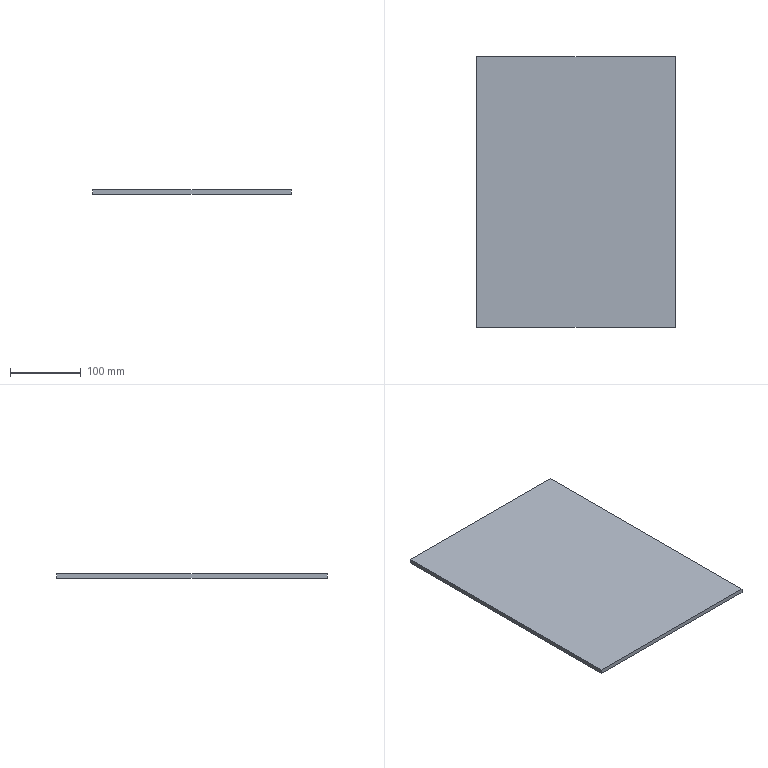Part | STEP file | Drawer | 1 solid | 6 faces | box 280 x 382 x 6 mm | volume 641760 mm3 | plane 6
STEP:
#1=CARTESIAN_POINT('',(0.,0.,0.));
#2=DIRECTION('',(0.,0.,1.));
#3=DIRECTION('',(1.,0.,0.));
#4=AXIS2_PLACEMENT_3D('',#1,#2,#3);
#5=CARTESIAN_POINT('',(-140.,191.,0.));
#6=VERTEX_POINT('',#5);
#7=CARTESIAN_POINT('',(-140.,191.,6.));
#8=VERTEX_POINT('',#7);
#9=CARTESIAN_POINT('',(-140.,191.,0.));
#10=DIRECTION('',(0.,0.,1.));
#11=VECTOR('',#10,1.);
#12=LINE('',#9,#11);
#13=CARTESIAN_POINT('',(-140.,191.,0.));
#14=DIRECTION('',(1.,0.,0.));
#15=DIRECTION('',(0.,-1.,0.));
#16=AXIS2_PLACEMENT_3D('',#13,#14,#15);
#17=PLANE('',#16);
#18=CARTESIAN_POINT('',(0.,0.));
#19=DIRECTION('',(0.,-1.));
#20=VECTOR('',#19,1.);
#21=LINE('',#18,#20);
#22=(GEOMETRIC_REPRESENTATION_CONTEXT(2)PARAMETRIC_REPRESENTATION_CONTEXT()REPRESENTATION_CONTEXT('',''));
#23=DEFINITIONAL_REPRESENTATION('',(#21),#22);
#24=PCURVE('',#17,#23);
#25=CARTESIAN_POINT('',(140.,191.,0.));
#26=DIRECTION('',(0.,-1.,0.));
#27=DIRECTION('',(-1.,0.,0.));
#28=AXIS2_PLACEMENT_3D('',#25,#26,#27);
#29=PLANE('',#28);
#30=CARTESIAN_POINT('',(280.,0.));
#31=DIRECTION('',(0.,-1.));
#32=VECTOR('',#31,1.);
#33=LINE('',#30,#32);
#34=(GEOMETRIC_REPRESENTATION_CONTEXT(2)PARAMETRIC_REPRESENTATION_CONTEXT()REPRESENTATION_CONTEXT('',''));
#35=DEFINITIONAL_REPRESENTATION('',(#33),#34);
#36=PCURVE('',#29,#35);
#37=SURFACE_CURVE('',#12,(#24,#36),.PCURVE_S1.);
#38=EDGE_CURVE('',#6,#8,#37,.T.);
#39=ORIENTED_EDGE('',*,*,#38,.T.);
#40=CARTESIAN_POINT('',(-140.,-191.,6.));
#41=VERTEX_POINT('',#40);
#42=CARTESIAN_POINT('',(-140.,191.,6.));
#43=DIRECTION('',(0.,-1.,0.));
#44=VECTOR('',#43,1.);
#45=LINE('',#42,#44);
#46=CARTESIAN_POINT('',(0.,-6.));
#47=DIRECTION('',(1.,0.));
#48=VECTOR('',#47,1.);
#49=LINE('',#46,#48);
#50=(GEOMETRIC_REPRESENTATION_CONTEXT(2)PARAMETRIC_REPRESENTATION_CONTEXT()REPRESENTATION_CONTEXT('',''));
#51=DEFINITIONAL_REPRESENTATION('',(#49),#50);
#52=PCURVE('',#17,#51);
#53=CARTESIAN_POINT('',(0.,0.,6.));
#54=DIRECTION('',(0.,0.,1.));
#55=DIRECTION('',(1.,0.,0.));
#56=AXIS2_PLACEMENT_3D('',#53,#54,#55);
#57=PLANE('',#56);
#58=CARTESIAN_POINT('',(-140.,191.));
#59=DIRECTION('',(0.,-1.));
#60=VECTOR('',#59,1.);
#61=LINE('',#58,#60);
#62=(GEOMETRIC_REPRESENTATION_CONTEXT(2)PARAMETRIC_REPRESENTATION_CONTEXT()REPRESENTATION_CONTEXT('',''));
#63=DEFINITIONAL_REPRESENTATION('',(#61),#62);
#64=PCURVE('',#57,#63);
#65=SURFACE_CURVE('',#45,(#52,#64),.PCURVE_S1.);
#66=EDGE_CURVE('',#8,#41,#65,.T.);
#67=ORIENTED_EDGE('',*,*,#66,.T.);
#68=CARTESIAN_POINT('',(-140.,-191.,0.));
#69=VERTEX_POINT('',#68);
#70=CARTESIAN_POINT('',(-140.,-191.,0.));
#71=DIRECTION('',(0.,0.,1.));
#72=VECTOR('',#71,1.);
#73=LINE('',#70,#72);
#74=CARTESIAN_POINT('',(382.,0.));
#75=DIRECTION('',(0.,-1.));
#76=VECTOR('',#75,1.);
#77=LINE('',#74,#76);
#78=(GEOMETRIC_REPRESENTATION_CONTEXT(2)PARAMETRIC_REPRESENTATION_CONTEXT()REPRESENTATION_CONTEXT('',''));
#79=DEFINITIONAL_REPRESENTATION('',(#77),#78);
#80=PCURVE('',#17,#79);
#81=CARTESIAN_POINT('',(-140.,-191.,0.));
#82=DIRECTION('',(0.,1.,0.));
#83=DIRECTION('',(1.,0.,0.));
#84=AXIS2_PLACEMENT_3D('',#81,#82,#83);
#85=PLANE('',#84);
#86=CARTESIAN_POINT('',(0.,0.));
#87=DIRECTION('',(0.,-1.));
#88=VECTOR('',#87,1.);
#89=LINE('',#86,#88);
#90=(GEOMETRIC_REPRESENTATION_CONTEXT(2)PARAMETRIC_REPRESENTATION_CONTEXT()REPRESENTATION_CONTEXT('',''));
#91=DEFINITIONAL_REPRESENTATION('',(#89),#90);
#92=PCURVE('',#85,#91);
#93=SURFACE_CURVE('',#73,(#80,#92),.PCURVE_S1.);
#94=EDGE_CURVE('',#69,#41,#93,.T.);
#95=ORIENTED_EDGE('',*,*,#94,.F.);
#96=CARTESIAN_POINT('',(-140.,191.,0.));
#97=DIRECTION('',(0.,-1.,0.));
#98=VECTOR('',#97,1.);
#99=LINE('',#96,#98);
#100=CARTESIAN_POINT('',(0.,0.));
#101=DIRECTION('',(1.,0.));
#102=VECTOR('',#101,1.);
#103=LINE('',#100,#102);
#104=(GEOMETRIC_REPRESENTATION_CONTEXT(2)PARAMETRIC_REPRESENTATION_CONTEXT()REPRESENTATION_CONTEXT('',''));
#105=DEFINITIONAL_REPRESENTATION('',(#103),#104);
#106=PCURVE('',#17,#105);
#107=CARTESIAN_POINT('',(0.,0.,0.));
#108=DIRECTION('',(0.,0.,1.));
#109=DIRECTION('',(1.,0.,0.));
#110=AXIS2_PLACEMENT_3D('',#107,#108,#109);
#111=PLANE('',#110);
#112=CARTESIAN_POINT('',(-140.,191.));
#113=DIRECTION('',(0.,-1.));
#114=VECTOR('',#113,1.);
#115=LINE('',#112,#114);
#116=(GEOMETRIC_REPRESENTATION_CONTEXT(2)PARAMETRIC_REPRESENTATION_CONTEXT()REPRESENTATION_CONTEXT('',''));
#117=DEFINITIONAL_REPRESENTATION('',(#115),#116);
#118=PCURVE('',#111,#117);
#119=SURFACE_CURVE('',#99,(#106,#118),.PCURVE_S1.);
#120=EDGE_CURVE('',#6,#69,#119,.T.);
#121=ORIENTED_EDGE('',*,*,#120,.F.);
#122=EDGE_LOOP('',(#39,#67,#95,#121));
#123=FACE_BOUND('',#122,.F.);
#124=ADVANCED_FACE('',(#123),#17,.F.);
#125=ORIENTED_EDGE('',*,*,#94,.T.);
#126=CARTESIAN_POINT('',(140.,-191.,6.));
#127=VERTEX_POINT('',#126);
#128=CARTESIAN_POINT('',(-140.,-191.,6.));
#129=DIRECTION('',(1.,0.,0.));
#130=VECTOR('',#129,1.);
#131=LINE('',#128,#130);
#132=CARTESIAN_POINT('',(0.,-6.));
#133=DIRECTION('',(1.,0.));
#134=VECTOR('',#133,1.);
#135=LINE('',#132,#134);
#136=(GEOMETRIC_REPRESENTATION_CONTEXT(2)PARAMETRIC_REPRESENTATION_CONTEXT()REPRESENTATION_CONTEXT('',''));
#137=DEFINITIONAL_REPRESENTATION('',(#135),#136);
#138=PCURVE('',#85,#137);
#139=CARTESIAN_POINT('',(-140.,-191.));
#140=DIRECTION('',(1.,0.));
#141=VECTOR('',#140,1.);
#142=LINE('',#139,#141);
#143=(GEOMETRIC_REPRESENTATION_CONTEXT(2)PARAMETRIC_REPRESENTATION_CONTEXT()REPRESENTATION_CONTEXT('',''));
#144=DEFINITIONAL_REPRESENTATION('',(#142),#143);
#145=PCURVE('',#57,#144);
#146=SURFACE_CURVE('',#131,(#138,#145),.PCURVE_S1.);
#147=EDGE_CURVE('',#41,#127,#146,.T.);
#148=ORIENTED_EDGE('',*,*,#147,.T.);
#149=CARTESIAN_POINT('',(140.,-191.,0.));
#150=VERTEX_POINT('',#149);
#151=CARTESIAN_POINT('',(140.,-191.,0.));
#152=DIRECTION('',(0.,0.,1.));
#153=VECTOR('',#152,1.);
#154=LINE('',#151,#153);
#155=CARTESIAN_POINT('',(280.,0.));
#156=DIRECTION('',(0.,-1.));
#157=VECTOR('',#156,1.);
#158=LINE('',#155,#157);
#159=(GEOMETRIC_REPRESENTATION_CONTEXT(2)PARAMETRIC_REPRESENTATION_CONTEXT()REPRESENTATION_CONTEXT('',''));
#160=DEFINITIONAL_REPRESENTATION('',(#158),#159);
#161=PCURVE('',#85,#160);
#162=CARTESIAN_POINT('',(140.,-191.,0.));
#163=DIRECTION('',(-1.,0.,0.));
#164=DIRECTION('',(0.,1.,0.));
#165=AXIS2_PLACEMENT_3D('',#162,#163,#164);
#166=PLANE('',#165);
#167=CARTESIAN_POINT('',(0.,0.));
#168=DIRECTION('',(0.,-1.));
#169=VECTOR('',#168,1.);
#170=LINE('',#167,#169);
#171=(GEOMETRIC_REPRESENTATION_CONTEXT(2)PARAMETRIC_REPRESENTATION_CONTEXT()REPRESENTATION_CONTEXT('',''));
#172=DEFINITIONAL_REPRESENTATION('',(#170),#171);
#173=PCURVE('',#166,#172);
#174=SURFACE_CURVE('',#154,(#161,#173),.PCURVE_S1.);
#175=EDGE_CURVE('',#150,#127,#174,.T.);
#176=ORIENTED_EDGE('',*,*,#175,.F.);
#177=CARTESIAN_POINT('',(-140.,-191.,0.));
#178=DIRECTION('',(1.,0.,0.));
#179=VECTOR('',#178,1.);
#180=LINE('',#177,#179);
#181=CARTESIAN_POINT('',(0.,0.));
#182=DIRECTION('',(1.,0.));
#183=VECTOR('',#182,1.);
#184=LINE('',#181,#183);
#185=(GEOMETRIC_REPRESENTATION_CONTEXT(2)PARAMETRIC_REPRESENTATION_CONTEXT()REPRESENTATION_CONTEXT('',''));
#186=DEFINITIONAL_REPRESENTATION('',(#184),#185);
#187=PCURVE('',#85,#186);
#188=CARTESIAN_POINT('',(-140.,-191.));
#189=DIRECTION('',(1.,0.));
#190=VECTOR('',#189,1.);
#191=LINE('',#188,#190);
#192=(GEOMETRIC_REPRESENTATION_CONTEXT(2)PARAMETRIC_REPRESENTATION_CONTEXT()REPRESENTATION_CONTEXT('',''));
#193=DEFINITIONAL_REPRESENTATION('',(#191),#192);
#194=PCURVE('',#111,#193);
#195=SURFACE_CURVE('',#180,(#187,#194),.PCURVE_S1.);
#196=EDGE_CURVE('',#69,#150,#195,.T.);
#197=ORIENTED_EDGE('',*,*,#196,.F.);
#198=EDGE_LOOP('',(#125,#148,#176,#197));
#199=FACE_BOUND('',#198,.F.);
#200=ADVANCED_FACE('',(#199),#85,.F.);
#201=ORIENTED_EDGE('',*,*,#175,.T.);
#202=CARTESIAN_POINT('',(140.,191.,6.));
#203=VERTEX_POINT('',#202);
#204=CARTESIAN_POINT('',(140.,-191.,6.));
#205=DIRECTION('',(0.,1.,0.));
#206=VECTOR('',#205,1.);
#207=LINE('',#204,#206);
#208=CARTESIAN_POINT('',(0.,-6.));
#209=DIRECTION('',(1.,0.));
#210=VECTOR('',#209,1.);
#211=LINE('',#208,#210);
#212=(GEOMETRIC_REPRESENTATION_CONTEXT(2)PARAMETRIC_REPRESENTATION_CONTEXT()REPRESENTATION_CONTEXT('',''));
#213=DEFINITIONAL_REPRESENTATION('',(#211),#212);
#214=PCURVE('',#166,#213);
#215=CARTESIAN_POINT('',(140.,-191.));
#216=DIRECTION('',(0.,1.));
#217=VECTOR('',#216,1.);
#218=LINE('',#215,#217);
#219=(GEOMETRIC_REPRESENTATION_CONTEXT(2)PARAMETRIC_REPRESENTATION_CONTEXT()REPRESENTATION_CONTEXT('',''));
#220=DEFINITIONAL_REPRESENTATION('',(#218),#219);
#221=PCURVE('',#57,#220);
#222=SURFACE_CURVE('',#207,(#214,#221),.PCURVE_S1.);
#223=EDGE_CURVE('',#127,#203,#222,.T.);
#224=ORIENTED_EDGE('',*,*,#223,.T.);
#225=CARTESIAN_POINT('',(140.,191.,0.));
#226=VERTEX_POINT('',#225);
#227=CARTESIAN_POINT('',(140.,191.,0.));
#228=DIRECTION('',(0.,0.,1.));
#229=VECTOR('',#228,1.);
#230=LINE('',#227,#229);
#231=CARTESIAN_POINT('',(382.,0.));
#232=DIRECTION('',(0.,-1.));
#233=VECTOR('',#232,1.);
#234=LINE('',#231,#233);
#235=(GEOMETRIC_REPRESENTATION_CONTEXT(2)PARAMETRIC_REPRESENTATION_CONTEXT()REPRESENTATION_CONTEXT('',''));
#236=DEFINITIONAL_REPRESENTATION('',(#234),#235);
#237=PCURVE('',#166,#236);
#238=CARTESIAN_POINT('',(0.,0.));
#239=DIRECTION('',(0.,-1.));
#240=VECTOR('',#239,1.);
#241=LINE('',#238,#240);
#242=(GEOMETRIC_REPRESENTATION_CONTEXT(2)PARAMETRIC_REPRESENTATION_CONTEXT()REPRESENTATION_CONTEXT('',''));
#243=DEFINITIONAL_REPRESENTATION('',(#241),#242);
#244=PCURVE('',#29,#243);
#245=SURFACE_CURVE('',#230,(#237,#244),.PCURVE_S1.);
#246=EDGE_CURVE('',#226,#203,#245,.T.);
#247=ORIENTED_EDGE('',*,*,#246,.F.);
#248=CARTESIAN_POINT('',(140.,-191.,0.));
#249=DIRECTION('',(0.,1.,0.));
#250=VECTOR('',#249,1.);
#251=LINE('',#248,#250);
#252=CARTESIAN_POINT('',(0.,0.));
#253=DIRECTION('',(1.,0.));
#254=VECTOR('',#253,1.);
#255=LINE('',#252,#254);
#256=(GEOMETRIC_REPRESENTATION_CONTEXT(2)PARAMETRIC_REPRESENTATION_CONTEXT()REPRESENTATION_CONTEXT('',''));
#257=DEFINITIONAL_REPRESENTATION('',(#255),#256);
#258=PCURVE('',#166,#257);
#259=CARTESIAN_POINT('',(140.,-191.));
#260=DIRECTION('',(0.,1.));
#261=VECTOR('',#260,1.);
#262=LINE('',#259,#261);
#263=(GEOMETRIC_REPRESENTATION_CONTEXT(2)PARAMETRIC_REPRESENTATION_CONTEXT()REPRESENTATION_CONTEXT('',''));
#264=DEFINITIONAL_REPRESENTATION('',(#262),#263);
#265=PCURVE('',#111,#264);
#266=SURFACE_CURVE('',#251,(#258,#265),.PCURVE_S1.);
#267=EDGE_CURVE('',#150,#226,#266,.T.);
#268=ORIENTED_EDGE('',*,*,#267,.F.);
#269=EDGE_LOOP('',(#201,#224,#247,#268));
#270=FACE_BOUND('',#269,.F.);
#271=ADVANCED_FACE('',(#270),#166,.F.);
#272=ORIENTED_EDGE('',*,*,#246,.T.);
#273=CARTESIAN_POINT('',(140.,191.,6.));
#274=DIRECTION('',(-1.,0.,0.));
#275=VECTOR('',#274,1.);
#276=LINE('',#273,#275);
#277=CARTESIAN_POINT('',(0.,-6.));
#278=DIRECTION('',(1.,0.));
#279=VECTOR('',#278,1.);
#280=LINE('',#277,#279);
#281=(GEOMETRIC_REPRESENTATION_CONTEXT(2)PARAMETRIC_REPRESENTATION_CONTEXT()REPRESENTATION_CONTEXT('',''));
#282=DEFINITIONAL_REPRESENTATION('',(#280),#281);
#283=PCURVE('',#29,#282);
#284=CARTESIAN_POINT('',(140.,191.));
#285=DIRECTION('',(-1.,0.));
#286=VECTOR('',#285,1.);
#287=LINE('',#284,#286);
#288=(GEOMETRIC_REPRESENTATION_CONTEXT(2)PARAMETRIC_REPRESENTATION_CONTEXT()REPRESENTATION_CONTEXT('',''));
#289=DEFINITIONAL_REPRESENTATION('',(#287),#288);
#290=PCURVE('',#57,#289);
#291=SURFACE_CURVE('',#276,(#283,#290),.PCURVE_S1.);
#292=EDGE_CURVE('',#203,#8,#291,.T.);
#293=ORIENTED_EDGE('',*,*,#292,.T.);
#294=ORIENTED_EDGE('',*,*,#38,.F.);
#295=CARTESIAN_POINT('',(140.,191.,0.));
#296=DIRECTION('',(-1.,0.,0.));
#297=VECTOR('',#296,1.);
#298=LINE('',#295,#297);
#299=CARTESIAN_POINT('',(0.,0.));
#300=DIRECTION('',(1.,0.));
#301=VECTOR('',#300,1.);
#302=LINE('',#299,#301);
#303=(GEOMETRIC_REPRESENTATION_CONTEXT(2)PARAMETRIC_REPRESENTATION_CONTEXT()REPRESENTATION_CONTEXT('',''));
#304=DEFINITIONAL_REPRESENTATION('',(#302),#303);
#305=PCURVE('',#29,#304);
#306=CARTESIAN_POINT('',(140.,191.));
#307=DIRECTION('',(-1.,0.));
#308=VECTOR('',#307,1.);
#309=LINE('',#306,#308);
#310=(GEOMETRIC_REPRESENTATION_CONTEXT(2)PARAMETRIC_REPRESENTATION_CONTEXT()REPRESENTATION_CONTEXT('',''));
#311=DEFINITIONAL_REPRESENTATION('',(#309),#310);
#312=PCURVE('',#111,#311);
#313=SURFACE_CURVE('',#298,(#305,#312),.PCURVE_S1.);
#314=EDGE_CURVE('',#226,#6,#313,.T.);
#315=ORIENTED_EDGE('',*,*,#314,.F.);
#316=EDGE_LOOP('',(#272,#293,#294,#315));
#317=FACE_BOUND('',#316,.F.);
#318=ADVANCED_FACE('',(#317),#29,.F.);
#319=ORIENTED_EDGE('',*,*,#120,.T.);
#320=ORIENTED_EDGE('',*,*,#196,.T.);
#321=ORIENTED_EDGE('',*,*,#267,.T.);
#322=ORIENTED_EDGE('',*,*,#314,.T.);
#323=EDGE_LOOP('',(#319,#320,#321,#322));
#324=FACE_BOUND('',#323,.F.);
#325=ADVANCED_FACE('',(#324),#111,.F.);
#326=ORIENTED_EDGE('',*,*,#66,.T.);
#327=ORIENTED_EDGE('',*,*,#147,.T.);
#328=ORIENTED_EDGE('',*,*,#223,.T.);
#329=ORIENTED_EDGE('',*,*,#292,.T.);
#330=EDGE_LOOP('',(#326,#327,#328,#329));
#331=FACE_BOUND('',#330,.T.);
#332=ADVANCED_FACE('',(#331),#57,.T.);
#333=CLOSED_SHELL('',(#124,#200,#271,#318,#325,#332));
#334=MANIFOLD_SOLID_BREP('',#333);
#335=(LENGTH_UNIT()NAMED_UNIT(*)SI_UNIT(.MILLI.,.METRE.));
#336=UNCERTAINTY_MEASURE_WITH_UNIT(LENGTH_MEASURE(0.0000001),#335,'','');
#337=(NAMED_UNIT(*)PLANE_ANGLE_UNIT()SI_UNIT($,.RADIAN.));
#338=(NAMED_UNIT(*)SI_UNIT($,.STERADIAN.)SOLID_ANGLE_UNIT());
#339=(GEOMETRIC_REPRESENTATION_CONTEXT(3)GLOBAL_UNCERTAINTY_ASSIGNED_CONTEXT((#336))GLOBAL_UNIT_ASSIGNED_CONTEXT((#335,#337,#338))REPRESENTATION_CONTEXT('',''));
#340=ADVANCED_BREP_SHAPE_REPRESENTATION('',(#4,#334),#339);